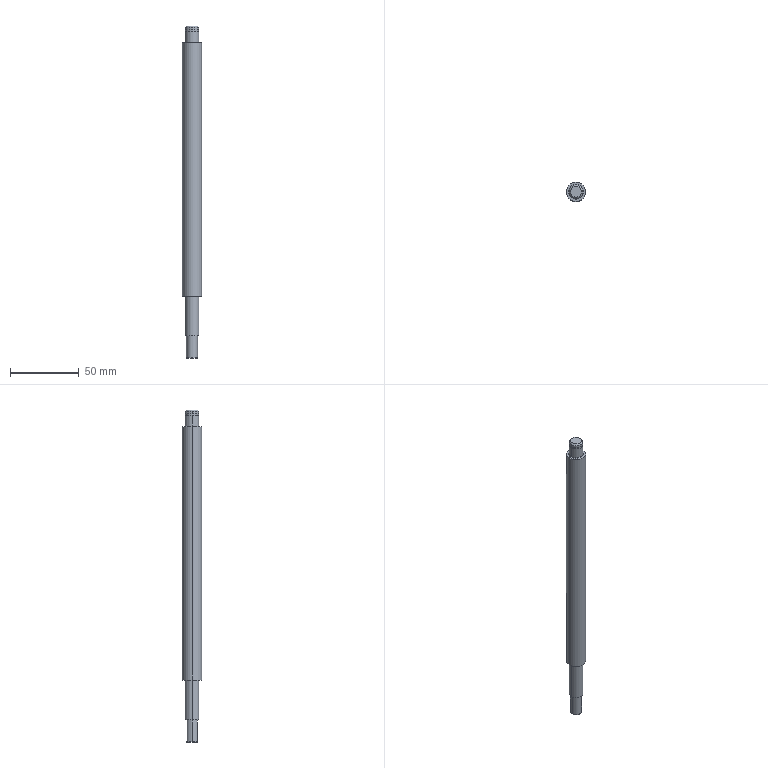Part | STEP file | 001-003-LHC07-D14-L241-S16 | 1 solid | 27 faces | box 14 x 14 x 241 mm | volume 32328 mm3 | cylinder 12 | plane 7 | cone 4 | torus 4 | commonest cylinder face diameters 10 x6 8 x2 9.6 x2 14 x2